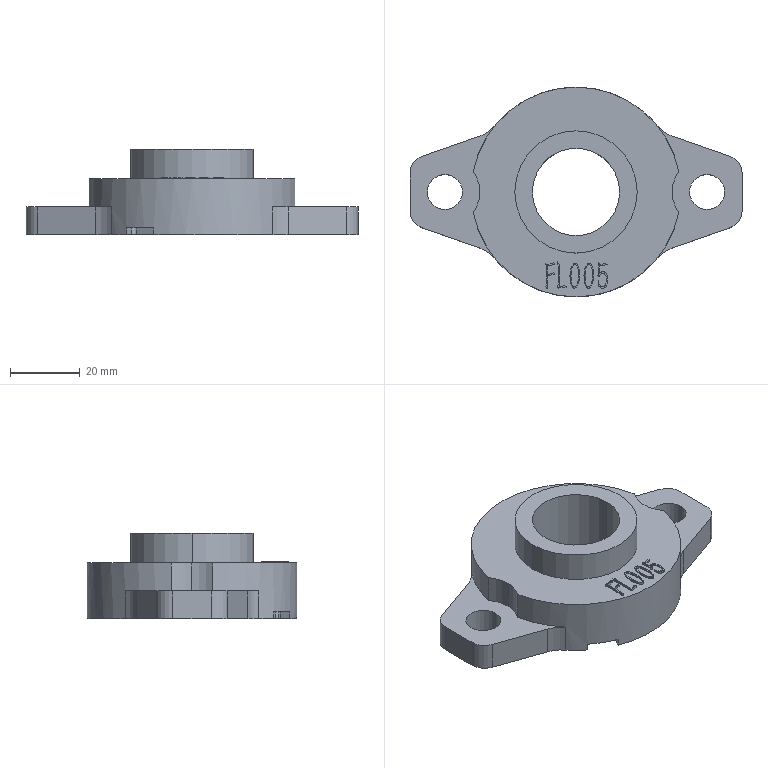Part | SolidWorks | features ICE 7, Fillet 3, MirrorPattern 2, Extrusion 1, HoleWzd 1, RefAxis 1 | 1 solid | 150 faces | box 95 x 60 x 24.5 mm | volume 44207 mm3 | plane 74 | spline 48 | cylinder 28 | commonest cylinder face diameters 10 x8 20 x7 2 x5 25 x2 35 x2 50 x2